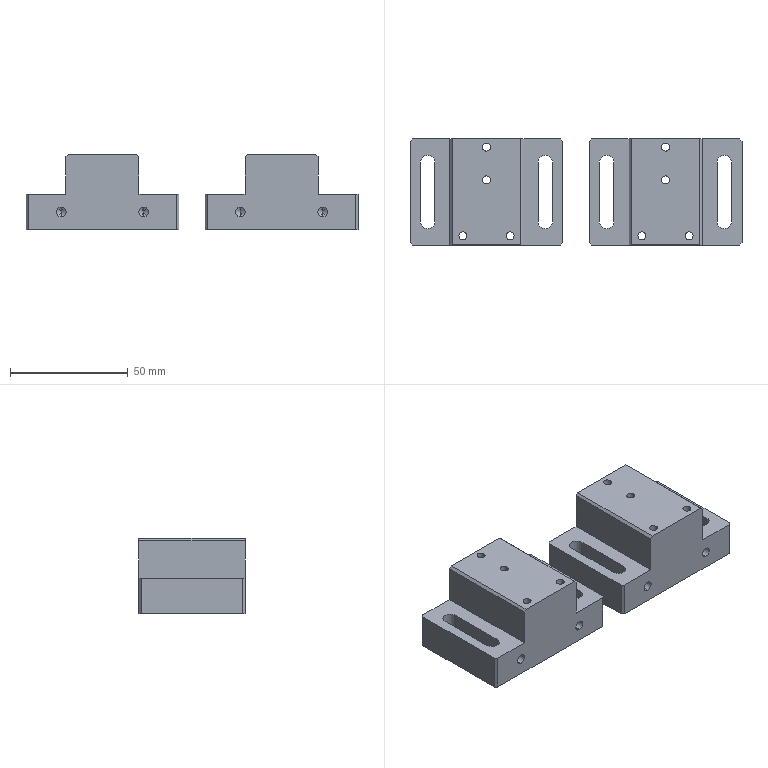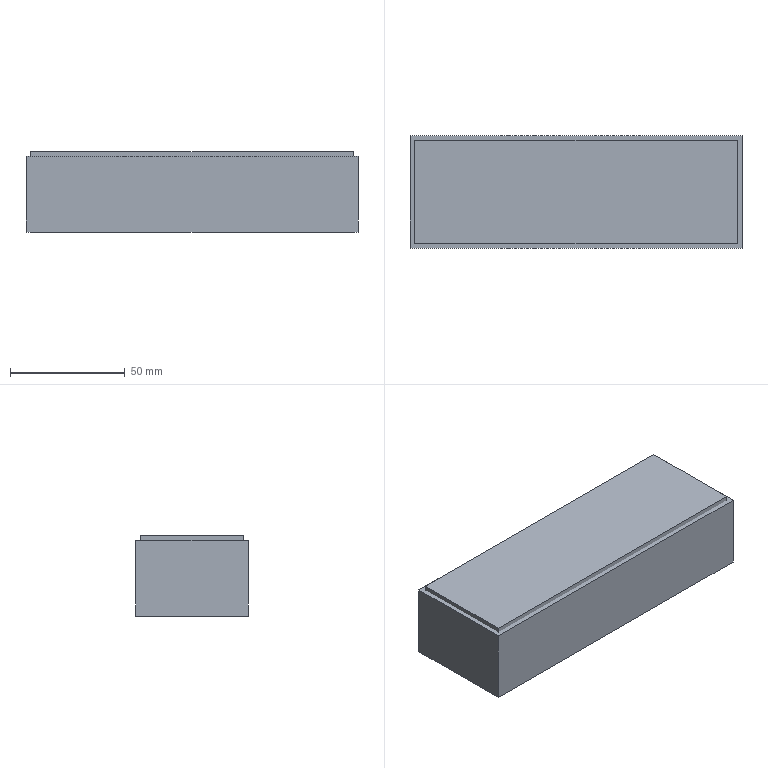CAM job | NX | 3-axis milling, drilling | part box 140.92 x 45 x 32 mm | stock box 144.92 x 49 x 35 mm
Tools:
number,name,description,diameter,corner_radius,flute_length,length,flutes
19,D80,Milling Tool-5 Parameters,80.0,0.0,50.0,75.0,2
15,D10,Milling Tool-5 Parameters,10.0,0.0,50.0,75.0,2
14,D10JING,Milling Tool-5 Parameters,10.0,0.0,50.0,75.0,2
11,D4,Milling Tool-5 Parameters,4.0,0.0,50.0,75.0,2
1,D6A45,Milling Tool-5 Parameters,6.0,0.0,50.0,75.0,2
16,3.4ZT,Drilling Tool,3.4,0.0,35.0,50.0,2
17,6.0ZT,Drilling Tool,6.0,0.0,35.0,50.0,2
Operations:
program,operation,operation_type,tool,method,geometry_group,spindle_rpm,surface_speed,feed_per_tooth,feed_cut,feed_plunge,cut_length_mm,path_length_mm,cut_time_min,machine_time_min
1,FLOOR_WALL,VolumeBased25DMillingOperation,D80,METHOD,A,6500.0,1633.0,0.1154,1500.0,100.0,236.92,290.92,0.1579,0.1633
1,ZLEVEL_PROFILE,ZLevelMilling,D10,METHOD,A,9500.0,298.0,0.1579,3000.0,1000.0,16573.762,16838.299,5.588,5.615
1,FLOOR_WALL_1,VolumeBased25DMillingOperation,D10,METHOD,A,9500.0,298.0,0.1842,3500.0,1000.0,13826.974,15058.502,4.411,4.534
1,FLOOR_WALL_1_COPY,VolumeBased25DMillingOperation,D10JING,METHOD,A,9500.0,298.0,0.0789,1500.0,1000.0,1206.451,1704.513,0.8143,0.8641
1,ZLEVEL_PROFILE_1,ZLevelMilling,D10JING,METHOD,A,9500.0,298.0,0.0789,1500.0,1000.0,1270.557,1737.558,0.8511,0.8978
1,DRILLING,Operation,D6A45,METHOD,A,9500.0,179.0,0.0132,250.0,0.0,38.4,334.563,0.1536,0.1832
1,DRILLING_COPY_COPY,Operation,3.4ZT,METHOD,A,2000.0,21.0,0.0375,150.0,0.0,152.972,563.707,1.02,1.061
1,PLANAR_MILL_COPY,PlanarMilling,D6A45,METHOD,A,9500.0,179.0,0.0658,1250.0,100.0,398.089,1189.923,0.3185,0.3977
1,PLANAR_MILL_COPY_COPY,PlanarMilling,D6A45,METHOD,A,9500.0,179.0,0.0658,1250.0,100.0,200.378,549.378,0.1603,0.1952
1,PLANAR_MILL_COPY_COPY_1,PlanarMilling,D6A45,METHOD,A,9500.0,179.0,0.0658,1250.0,800.0,606.947,1699.082,0.4974,0.6066
2,FLOOR_WALL_COPY,VolumeBased25DMillingOperation,D80,METHOD,B,6500.0,1633.0,0.1154,1500.0,100.0,698.76,1308.601,0.4658,0.5268
2,ZLEVEL_PROFILE_COPY,ZLevelMilling,D4,METHOD,B,9500.0,119.0,0.0711,1350.0,1000.0,10155.997,10576.109,7.56,7.602
2,DRILLING_COPY,Operation,D6A45,METHOD,B,9500.0,179.0,0.0132,250.0,0.0,38.4,334.563,0.1536,0.1832
2,DRILLING_COPY_COPY_COPY,Operation,6.0ZT,METHOD,B,2000.0,21.0,0.0375,150.0,0.0,185.621,629.005,1.238,1.282
2,PLANAR_MILL_COPY_COPY_2,PlanarMilling,D6A45,METHOD,B,9500.0,179.0,0.0658,1250.0,100.0,878.662,2028.013,0.7029,0.8179